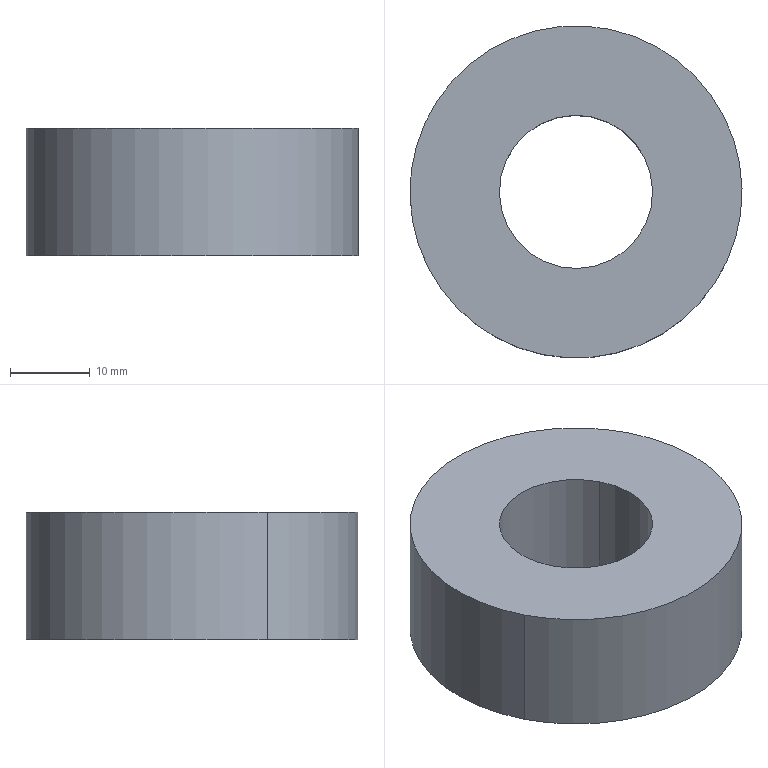Part | SolidWorks | features BaseBody 1 | 1 solid | 6 faces | box 41.6 x 41.6 x 16 mm | volume 17114 mm3 | cylinder 4 | plane 2 | commonest cylinder face diameters 19.2 x2 41.6 x2
STEP:
#1=CARTESIAN_POINT('',(-327.735,-31.13,425.));
#2=VERTEX_POINT('',#1);
#3=CARTESIAN_POINT('',(-310.627,-22.415,425.));
#4=VERTEX_POINT('',#3);
#5=CARTESIAN_POINT('',(-319.181,-26.773,425.));
#6=DIRECTION('',(0.,0.,1.));
#7=DIRECTION('',(0.8911,0.4539,0.));
#8=AXIS2_PLACEMENT_3D('',#5,#6,#7);
#9=CIRCLE('',#8,9.6);
#10=EDGE_CURVE('',#2,#4,#9,.T.);
#11=ORIENTED_EDGE('',*,*,#10,.T.);
#12=CARTESIAN_POINT('',(-310.627,-22.415,409.));
#13=VERTEX_POINT('',#12);
#14=CARTESIAN_POINT('',(-310.627,-22.415,425.));
#15=DIRECTION('',(0.,0.,-1.));
#16=VECTOR('',#15,1000.);
#17=LINE('',#14,#16);
#18=EDGE_CURVE('',#4,#13,#17,.T.);
#19=ORIENTED_EDGE('',*,*,#18,.T.);
#20=CARTESIAN_POINT('',(-327.735,-31.13,409.));
#21=VERTEX_POINT('',#20);
#22=CARTESIAN_POINT('',(-319.181,-26.773,409.));
#23=DIRECTION('',(0.,0.,1.));
#24=DIRECTION('',(0.8911,0.4539,0.));
#25=AXIS2_PLACEMENT_3D('',#22,#23,#24);
#26=CIRCLE('',#25,9.6);
#27=EDGE_CURVE('',#21,#13,#26,.T.);
#28=ORIENTED_EDGE('',*,*,#27,.F.);
#29=CARTESIAN_POINT('',(-327.735,-31.13,425.));
#30=DIRECTION('',(0.,0.,-1.));
#31=VECTOR('',#30,1000.);
#32=LINE('',#29,#31);
#33=EDGE_CURVE('',#2,#21,#32,.T.);
#34=ORIENTED_EDGE('',*,*,#33,.F.);
#35=EDGE_LOOP('',(#11,#19,#28,#34));
#36=FACE_OUTER_BOUND('',#35,.T.);
#37=CARTESIAN_POINT('',(-319.181,-26.773,425.));
#38=DIRECTION('',(0.,0.,-1.));
#39=DIRECTION('',(-0.8911,-0.4539,0.));
#40=AXIS2_PLACEMENT_3D('',#37,#38,#39);
#41=CYLINDRICAL_SURFACE('',#40,9.6);
#42=ADVANCED_FACE('',(#36),#41,.F.);
#43=CARTESIAN_POINT('',(-300.647,-17.332,425.));
#44=VERTEX_POINT('',#43);
#45=CARTESIAN_POINT('',(-337.715,-36.213,425.));
#46=VERTEX_POINT('',#45);
#47=CARTESIAN_POINT('',(-319.181,-26.773,425.));
#48=DIRECTION('',(0.,0.,1.));
#49=DIRECTION('',(0.8911,0.4539,0.));
#50=AXIS2_PLACEMENT_3D('',#47,#48,#49);
#51=CIRCLE('',#50,20.8);
#52=EDGE_CURVE('',#44,#46,#51,.T.);
#53=ORIENTED_EDGE('',*,*,#52,.F.);
#54=CARTESIAN_POINT('',(-300.647,-17.332,409.));
#55=VERTEX_POINT('',#54);
#56=CARTESIAN_POINT('',(-300.647,-17.332,425.));
#57=DIRECTION('',(0.,0.,-1.));
#58=VECTOR('',#57,1000.);
#59=LINE('',#56,#58);
#60=EDGE_CURVE('',#44,#55,#59,.T.);
#61=ORIENTED_EDGE('',*,*,#60,.T.);
#62=CARTESIAN_POINT('',(-337.715,-36.213,409.));
#63=VERTEX_POINT('',#62);
#64=CARTESIAN_POINT('',(-319.181,-26.773,409.));
#65=DIRECTION('',(0.,0.,1.));
#66=DIRECTION('',(0.8911,0.4539,0.));
#67=AXIS2_PLACEMENT_3D('',#64,#65,#66);
#68=CIRCLE('',#67,20.8);
#69=EDGE_CURVE('',#55,#63,#68,.T.);
#70=ORIENTED_EDGE('',*,*,#69,.T.);
#71=CARTESIAN_POINT('',(-337.715,-36.213,425.));
#72=DIRECTION('',(0.,0.,-1.));
#73=VECTOR('',#72,1000.);
#74=LINE('',#71,#73);
#75=EDGE_CURVE('',#46,#63,#74,.T.);
#76=ORIENTED_EDGE('',*,*,#75,.F.);
#77=EDGE_LOOP('',(#53,#61,#70,#76));
#78=FACE_OUTER_BOUND('',#77,.T.);
#79=CARTESIAN_POINT('',(-319.181,-26.773,425.));
#80=DIRECTION('',(0.,0.,-1.));
#81=DIRECTION('',(-0.8911,-0.4539,0.));
#82=AXIS2_PLACEMENT_3D('',#79,#80,#81);
#83=CYLINDRICAL_SURFACE('',#82,20.8);
#84=ADVANCED_FACE('',(#78),#83,.T.);
#85=CARTESIAN_POINT('',(-319.181,-26.773,425.));
#86=DIRECTION('',(0.,0.,1.));
#87=DIRECTION('',(0.8911,0.4539,0.));
#88=AXIS2_PLACEMENT_3D('',#85,#86,#87);
#89=CIRCLE('',#88,20.8);
#90=EDGE_CURVE('',#46,#44,#89,.T.);
#91=ORIENTED_EDGE('',*,*,#90,.T.);
#92=ORIENTED_EDGE('',*,*,#52,.T.);
#93=EDGE_LOOP('',(#91,#92));
#94=FACE_OUTER_BOUND('',#93,.T.);
#95=ORIENTED_EDGE('',*,*,#10,.F.);
#96=CARTESIAN_POINT('',(-319.181,-26.773,425.));
#97=DIRECTION('',(0.,0.,1.));
#98=DIRECTION('',(0.8911,0.4539,0.));
#99=AXIS2_PLACEMENT_3D('',#96,#97,#98);
#100=CIRCLE('',#99,9.6);
#101=EDGE_CURVE('',#4,#2,#100,.T.);
#102=ORIENTED_EDGE('',*,*,#101,.F.);
#103=EDGE_LOOP('',(#95,#102));
#104=FACE_BOUND('',#103,.T.);
#105=CARTESIAN_POINT('',(-319.181,-26.773,425.));
#106=DIRECTION('',(0.,0.,1.));
#107=DIRECTION('',(0.8911,0.4539,0.));
#108=AXIS2_PLACEMENT_3D('',#105,#106,#107);
#109=PLANE('',#108);
#110=ADVANCED_FACE('',(#94,#104),#109,.T.);
#111=CARTESIAN_POINT('',(-319.181,-26.773,409.));
#112=DIRECTION('',(0.,0.,1.));
#113=DIRECTION('',(0.8911,0.4539,0.));
#114=AXIS2_PLACEMENT_3D('',#111,#112,#113);
#115=CIRCLE('',#114,20.8);
#116=EDGE_CURVE('',#63,#55,#115,.T.);
#117=ORIENTED_EDGE('',*,*,#116,.F.);
#118=ORIENTED_EDGE('',*,*,#69,.F.);
#119=EDGE_LOOP('',(#117,#118));
#120=FACE_OUTER_BOUND('',#119,.T.);
#121=ORIENTED_EDGE('',*,*,#27,.T.);
#122=CARTESIAN_POINT('',(-319.181,-26.773,409.));
#123=DIRECTION('',(0.,0.,1.));
#124=DIRECTION('',(0.8911,0.4539,0.));
#125=AXIS2_PLACEMENT_3D('',#122,#123,#124);
#126=CIRCLE('',#125,9.6);
#127=EDGE_CURVE('',#13,#21,#126,.T.);
#128=ORIENTED_EDGE('',*,*,#127,.T.);
#129=EDGE_LOOP('',(#121,#128));
#130=FACE_BOUND('',#129,.T.);
#131=CARTESIAN_POINT('',(-319.181,-26.773,409.));
#132=DIRECTION('',(0.,0.,1.));
#133=DIRECTION('',(0.8911,0.4539,0.));
#134=AXIS2_PLACEMENT_3D('',#131,#132,#133);
#135=PLANE('',#134);
#136=ADVANCED_FACE('',(#120,#130),#135,.F.);
#137=ORIENTED_EDGE('',*,*,#60,.F.);
#138=ORIENTED_EDGE('',*,*,#90,.F.);
#139=ORIENTED_EDGE('',*,*,#75,.T.);
#140=ORIENTED_EDGE('',*,*,#116,.T.);
#141=EDGE_LOOP('',(#137,#138,#139,#140));
#142=FACE_OUTER_BOUND('',#141,.T.);
#143=CARTESIAN_POINT('',(-319.181,-26.773,425.));
#144=DIRECTION('',(0.,0.,-1.));
#145=DIRECTION('',(-0.8911,-0.4539,0.));
#146=AXIS2_PLACEMENT_3D('',#143,#144,#145);
#147=CYLINDRICAL_SURFACE('',#146,20.8);
#148=ADVANCED_FACE('',(#142),#147,.T.);
#149=ORIENTED_EDGE('',*,*,#18,.F.);
#150=ORIENTED_EDGE('',*,*,#101,.T.);
#151=ORIENTED_EDGE('',*,*,#33,.T.);
#152=ORIENTED_EDGE('',*,*,#127,.F.);
#153=EDGE_LOOP('',(#149,#150,#151,#152));
#154=FACE_OUTER_BOUND('',#153,.T.);
#155=CARTESIAN_POINT('',(-319.181,-26.773,425.));
#156=DIRECTION('',(0.,0.,-1.));
#157=DIRECTION('',(-0.8911,-0.4539,0.));
#158=AXIS2_PLACEMENT_3D('',#155,#156,#157);
#159=CYLINDRICAL_SURFACE('',#158,9.6);
#160=ADVANCED_FACE('',(#154),#159,.F.);
#161=CLOSED_SHELL('',(#42,#84,#110,#136,#148,#160));
#162=MANIFOLD_SOLID_BREP('',#161);
#163=CARTESIAN_POINT('',(0.,0.,0.));
#164=DIRECTION('',(0.,0.,1.));
#165=DIRECTION('',(1.,0.,0.));
#166=AXIS2_PLACEMENT_3D('',#163,#164,#165);
#167=(LENGTH_UNIT()NAMED_UNIT(*)SI_UNIT(.MILLI.,.METRE.));
#168=UNCERTAINTY_MEASURE_WITH_UNIT(LENGTH_MEASURE(0.00001),#167,'','');
#169=(NAMED_UNIT(*)PLANE_ANGLE_UNIT()SI_UNIT($,.RADIAN.));
#170=(NAMED_UNIT(*)SI_UNIT($,.STERADIAN.)SOLID_ANGLE_UNIT());
#171=(GEOMETRIC_REPRESENTATION_CONTEXT(3)GLOBAL_UNCERTAINTY_ASSIGNED_CONTEXT((#168))GLOBAL_UNIT_ASSIGNED_CONTEXT((#167,#169,#170))REPRESENTATION_CONTEXT('',''));
#172=ADVANCED_BREP_SHAPE_REPRESENTATION('',(#162,#166),#171);